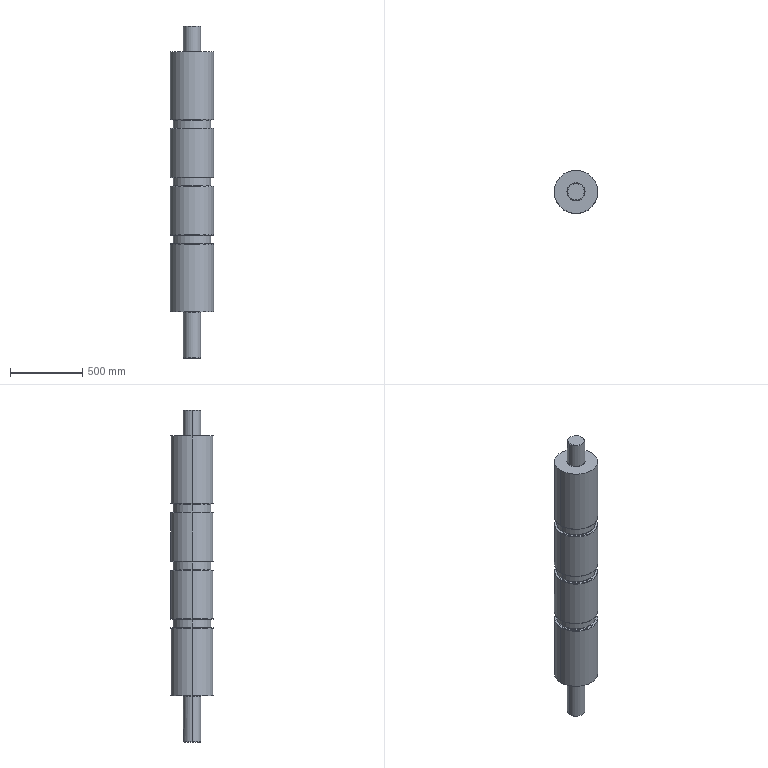Part | SolidWorks | features ICE 3, Chamfer 2, Extrusion 1, Fillet 1, LPattern 1, RefAxis 1, RevCut 1 | 1 solid | 65 faces | box 300 x 300 x 2300 mm | volume 129677535 mm3 | torus 24 | cylinder 18 | plane 14 | cone 9 | commonest cylinder face diameters 300 x8 260 x6 120 x4